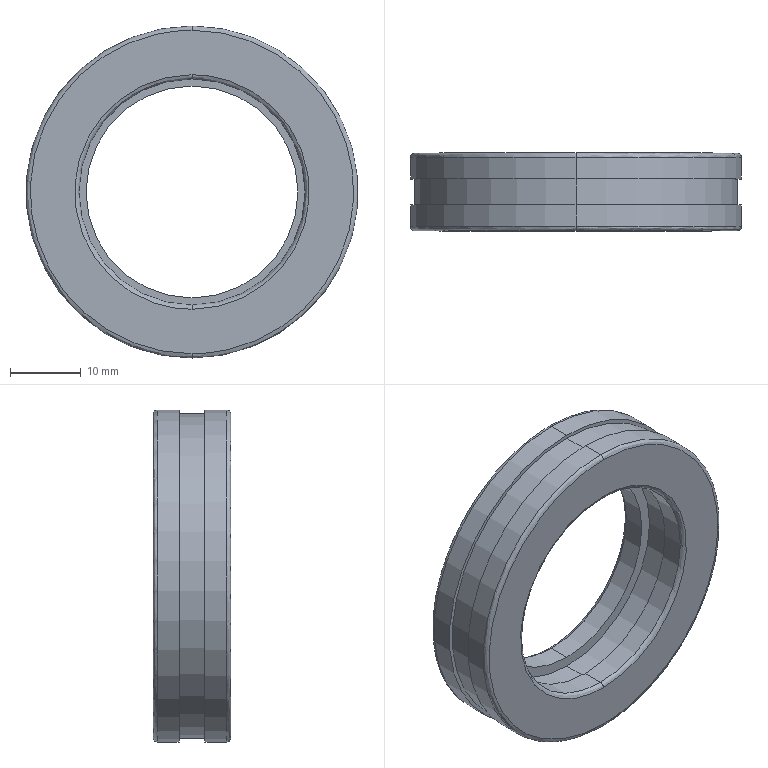Part | SolidWorks | features BaseBody 1 | 1 solid | 26 faces | box 47 x 11 x 47 mm | volume 10056 mm3 | cylinder 12 | spline 8 | plane 6 | commonest cylinder face diameters 47 x4 30 x2 32 x2 33.1 x2 45.9 x2
STEP:
#1=CARTESIAN_POINT('',(0.,10.4,-23.5));
#2=VERTEX_POINT('',#1);
#3=CARTESIAN_POINT('',(0.,10.4,23.5));
#4=VERTEX_POINT('',#3);
#5=CARTESIAN_POINT('',(0.,10.4,0.));
#6=DIRECTION('',(0.,1.,0.));
#7=DIRECTION('',(0.,0.,-1.));
#8=AXIS2_PLACEMENT_3D('',#5,#6,#7);
#9=CIRCLE('',#8,23.5);
#10=EDGE_CURVE('',#2,#4,#9,.T.);
#11=ORIENTED_EDGE('',*,*,#10,.T.);
#12=CARTESIAN_POINT('',(0.,11.,22.9));
#13=VERTEX_POINT('',#12);
#14=CARTESIAN_POINT('',(0.,10.4,22.9));
#15=DIRECTION('',(-1.,0.,0.));
#16=DIRECTION('',(0.,0.,1.));
#17=AXIS2_PLACEMENT_3D('',#14,#15,#16);
#18=CIRCLE('',#17,0.6);
#19=EDGE_CURVE('',#4,#13,#18,.T.);
#20=ORIENTED_EDGE('',*,*,#19,.T.);
#21=CARTESIAN_POINT('',(0.,11.,-22.9));
#22=VERTEX_POINT('',#21);
#23=CARTESIAN_POINT('',(0.,11.,-22.9));
#24=CARTESIAN_POINT('',(-0.7002,11.,-22.9));
#25=CARTESIAN_POINT('',(-1.746,11.,-22.852));
#26=CARTESIAN_POINT('',(-2.959,11.,-22.713));
#27=CARTESIAN_POINT('',(-3.564,11.,-22.622));
#28=CARTESIAN_POINT('',(-3.865,11.,-22.572));
#29=CARTESIAN_POINT('',(-4.016,11.,-22.545));
#30=CARTESIAN_POINT('',(-4.081,11.,-22.533));
#31=CARTESIAN_POINT('',(-4.124,11.,-22.526));
#32=CARTESIAN_POINT('',(-4.144,11.,-22.522));
#33=CARTESIAN_POINT('',(-4.897,11.,-22.383));
#34=CARTESIAN_POINT('',(-5.977,11.,-22.128));
#35=CARTESIAN_POINT('',(-7.212,11.,-21.74));
#36=CARTESIAN_POINT('',(-7.823,11.,-21.524));
#37=CARTESIAN_POINT('',(-8.127,11.,-21.41));
#38=CARTESIAN_POINT('',(-8.257,11.,-21.36));
#39=CARTESIAN_POINT('',(-8.343,11.,-21.326));
#40=CARTESIAN_POINT('',(-8.384,11.,-21.31));
#41=CARTESIAN_POINT('',(-9.149,11.,-21.007));
#42=CARTESIAN_POINT('',(-10.201,11.,-20.528));
#43=CARTESIAN_POINT('',(-11.382,11.,-19.878));
#44=CARTESIAN_POINT('',(-11.96,11.,-19.53));
#45=CARTESIAN_POINT('',(-12.206,11.,-19.376));
#46=CARTESIAN_POINT('',(-12.369,11.,-19.273));
#47=CARTESIAN_POINT('',(-12.448,11.,-19.221));
#48=CARTESIAN_POINT('',(-13.854,11.,-18.302));
#49=CARTESIAN_POINT('',(-15.075,11.,-17.31));
#50=CARTESIAN_POINT('',(-16.752,11.,-15.634));
#51=CARTESIAN_POINT('',(-17.542,11.,-14.757));
#52=CARTESIAN_POINT('',(-18.382,11.,-13.667));
#53=CARTESIAN_POINT('',(-18.782,11.,-13.105));
#54=CARTESIAN_POINT('',(-18.948,11.,-12.86));
#55=CARTESIAN_POINT('',(-19.059,11.,-12.696));
#56=CARTESIAN_POINT('',(-19.114,11.,-12.612));
#57=CARTESIAN_POINT('',(-19.591,11.,-11.884));
#58=CARTESIAN_POINT('',(-20.174,11.,-10.885));
#59=CARTESIAN_POINT('',(-20.763,11.,-9.673));
#60=CARTESIAN_POINT('',(-21.035,11.,-9.055));
#61=CARTESIAN_POINT('',(-21.166,11.,-8.743));
#62=CARTESIAN_POINT('',(-21.22,11.,-8.609));
#63=CARTESIAN_POINT('',(-21.256,11.,-8.519));
#64=CARTESIAN_POINT('',(-21.275,11.,-8.473));
#65=CARTESIAN_POINT('',(-21.565,11.,-7.739));
#66=CARTESIAN_POINT('',(-21.924,11.,-6.688));
#67=CARTESIAN_POINT('',(-22.251,11.,-5.436));
#68=CARTESIAN_POINT('',(-22.392,11.,-4.804));
#69=CARTESIAN_POINT('',(-22.457,11.,-4.486));
#70=CARTESIAN_POINT('',(-22.488,11.,-4.327));
#71=CARTESIAN_POINT('',(-22.501,11.,-4.258));
#72=CARTESIAN_POINT('',(-22.509,11.,-4.213));
#73=CARTESIAN_POINT('',(-22.514,11.,-4.188));
#74=CARTESIAN_POINT('',(-22.773,11.,-2.79));
#75=CARTESIAN_POINT('',(-22.9,11.,-1.4));
#76=CARTESIAN_POINT('',(-22.9,11.,0.7002));
#77=CARTESIAN_POINT('',(-22.852,11.,1.746));
#78=CARTESIAN_POINT('',(-22.713,11.,2.959));
#79=CARTESIAN_POINT('',(-22.622,11.,3.564));
#80=CARTESIAN_POINT('',(-22.572,11.,3.865));
#81=CARTESIAN_POINT('',(-22.545,11.,4.016));
#82=CARTESIAN_POINT('',(-22.533,11.,4.081));
#83=CARTESIAN_POINT('',(-22.526,11.,4.124));
#84=CARTESIAN_POINT('',(-22.522,11.,4.144));
#85=CARTESIAN_POINT('',(-22.383,11.,4.897));
#86=CARTESIAN_POINT('',(-22.128,11.,5.977));
#87=CARTESIAN_POINT('',(-21.74,11.,7.212));
#88=CARTESIAN_POINT('',(-21.524,11.,7.823));
#89=CARTESIAN_POINT('',(-21.41,11.,8.127));
#90=CARTESIAN_POINT('',(-21.36,11.,8.257));
#91=CARTESIAN_POINT('',(-21.326,11.,8.343));
#92=CARTESIAN_POINT('',(-21.31,11.,8.384));
#93=CARTESIAN_POINT('',(-21.007,11.,9.149));
#94=CARTESIAN_POINT('',(-20.528,11.,10.201));
#95=CARTESIAN_POINT('',(-19.878,11.,11.382));
#96=CARTESIAN_POINT('',(-19.53,11.,11.96));
#97=CARTESIAN_POINT('',(-19.376,11.,12.206));
#98=CARTESIAN_POINT('',(-19.273,11.,12.369));
#99=CARTESIAN_POINT('',(-19.221,11.,12.448));
#100=CARTESIAN_POINT('',(-18.302,11.,13.854));
#101=CARTESIAN_POINT('',(-17.31,11.,15.075));
#102=CARTESIAN_POINT('',(-15.634,11.,16.752));
#103=CARTESIAN_POINT('',(-14.757,11.,17.542));
#104=CARTESIAN_POINT('',(-13.667,11.,18.382));
#105=CARTESIAN_POINT('',(-13.105,11.,18.782));
#106=CARTESIAN_POINT('',(-12.86,11.,18.948));
#107=CARTESIAN_POINT('',(-12.696,11.,19.059));
#108=CARTESIAN_POINT('',(-12.612,11.,19.114));
#109=CARTESIAN_POINT('',(-11.884,11.,19.591));
#110=CARTESIAN_POINT('',(-10.885,11.,20.174));
#111=CARTESIAN_POINT('',(-9.673,11.,20.763));
#112=CARTESIAN_POINT('',(-9.055,11.,21.035));
#113=CARTESIAN_POINT('',(-8.743,11.,21.166));
#114=CARTESIAN_POINT('',(-8.609,11.,21.22));
#115=CARTESIAN_POINT('',(-8.519,11.,21.256));
#116=CARTESIAN_POINT('',(-8.473,11.,21.275));
#117=CARTESIAN_POINT('',(-7.739,11.,21.565));
#118=CARTESIAN_POINT('',(-6.688,11.,21.924));
#119=CARTESIAN_POINT('',(-5.436,11.,22.251));
#120=CARTESIAN_POINT('',(-4.804,11.,22.392));
#121=CARTESIAN_POINT('',(-4.486,11.,22.457));
#122=CARTESIAN_POINT('',(-4.327,11.,22.488));
#123=CARTESIAN_POINT('',(-4.258,11.,22.501));
#124=CARTESIAN_POINT('',(-4.213,11.,22.509));
#125=CARTESIAN_POINT('',(-4.188,11.,22.514));
#126=CARTESIAN_POINT('',(-2.79,11.,22.773));
#127=CARTESIAN_POINT('',(-1.4,11.,22.9));
#128=CARTESIAN_POINT('',(0.,11.,22.9));
#129=B_SPLINE_CURVE_WITH_KNOTS('',3,(#23,#24,#25,#26,#27,#28,#29,#30,#31,#32,#33,#34,#35,#36,#37,#38,#39,#40,#41,#42,#43,#44,#45,#46,#47,#48,#49,#50,#51,#52,#53,#54,#55,#56,#57,#58,#59,#60,#61,#62,#63,#64,#65,#66,#67,#68,#69,#70,#71,#72,#73,#74,#75,#76,#77,#78,#79,#80,#81,#82,#83,#84,#85,#86,#87,#88,#89,#90,#91,#92,#93,#94,#95,#96,#97,#98,#99,#100,#101,#102,#103,#104,#105,#106,#107,#108,#109,#110,#111,#112,#113,#114,#115,#116,#117,#118,#119,#120,#121,#122,#123,#124,#125,#126,#127,#128),.UNSPECIFIED.,.F.,.F.,(4,1,1,1,1,1,2,2,1,1,1,1,2,2,1,1,1,2,2,2,1,1,1,2,2,1,1,1,1,2,2,1,1,1,1,1,2,2,2,1,1,1,1,1,2,2,1,1,1,1,2,2,1,1,1,2,2,2,1,1,1,2,2,1,1,1,1,2,2,1,1,1,1,1,2,2,4),(0.,0.01563,0.02344,0.02734,0.0293,0.03027,0.03076,0.03125,0.04688,0.05469,0.05859,0.06055,0.06152,0.0625,0.07813,0.08594,0.08984,0.0918,0.09375,0.125,0.1406,0.1484,0.1523,0.1543,0.1563,0.1719,0.1797,0.1836,0.1855,0.1865,0.1875,0.2031,0.2109,0.2148,0.2168,0.2178,0.2183,0.2188,0.25,0.2656,0.2734,0.2773,0.2793,0.2803,0.2808,0.2813,0.2969,0.3047,0.3086,0.3105,0.3115,0.3125,0.3281,0.3359,0.3398,0.3418,0.3438,0.375,0.3906,0.3984,0.4023,0.4043,0.4063,0.4219,0.4297,0.4336,0.4355,0.4365,0.4375,0.4531,0.4609,0.4648,0.4668,0.4678,0.4683,0.4688,0.5),.UNSPECIFIED.);
#130=EDGE_CURVE('',#22,#13,#129,.T.);
#131=ORIENTED_EDGE('',*,*,#130,.F.);
#132=CARTESIAN_POINT('',(0.,10.4,-22.9));
#133=DIRECTION('',(1.,0.,0.));
#134=DIRECTION('',(0.,0.,-1.));
#135=AXIS2_PLACEMENT_3D('',#132,#133,#134);
#136=CIRCLE('',#135,0.6);
#137=EDGE_CURVE('',#2,#22,#136,.T.);
#138=ORIENTED_EDGE('',*,*,#137,.F.);
#139=EDGE_LOOP('',(#11,#20,#131,#138));
#140=FACE_OUTER_BOUND('',#139,.T.);
#141=CARTESIAN_POINT('',(0.,10.4,23.5));
#142=CARTESIAN_POINT('',(-47.,10.4,23.5));
#143=CARTESIAN_POINT('',(-47.,10.4,-23.5));
#144=CARTESIAN_POINT('',(0.,10.4,-23.5));
#145=CARTESIAN_POINT('',(0.,10.751,23.5));
#146=CARTESIAN_POINT('',(-47.,10.751,23.5));
#147=CARTESIAN_POINT('',(-47.,10.751,-23.5));
#148=CARTESIAN_POINT('',(0.,10.751,-23.5));
#149=CARTESIAN_POINT('',(0.,11.,23.251));
#150=CARTESIAN_POINT('',(-46.503,11.,23.251));
#151=CARTESIAN_POINT('',(-46.503,11.,-23.251));
#152=CARTESIAN_POINT('',(0.,11.,-23.251));
#153=CARTESIAN_POINT('',(0.,11.,22.9));
#154=CARTESIAN_POINT('',(-45.8,11.,22.9));
#155=CARTESIAN_POINT('',(-45.8,11.,-22.9));
#156=CARTESIAN_POINT('',(0.,11.,-22.9));
#157=(BOUNDED_SURFACE()B_SPLINE_SURFACE(3,3,((#141,#142,#143,#144),(#145,#146,#147,#148),(#149,#150,#151,#152),(#153,#154,#155,#156)),.UNSPECIFIED.,.F.,.F.,.F.)B_SPLINE_SURFACE_WITH_KNOTS((4,4),(4,4),(0.,1.),(0.,1.),.UNSPECIFIED.)GEOMETRIC_REPRESENTATION_ITEM()RATIONAL_B_SPLINE_SURFACE(((1.,0.3333,0.3333,1.),(0.8047,0.2682,0.2682,0.8047),(0.8047,0.2682,0.2682,0.8047),(1.,0.3333,0.3333,1.)))REPRESENTATION_ITEM('')SURFACE());
#158=ADVANCED_FACE('',(#140),#157,.T.);
#159=CARTESIAN_POINT('',(0.,11.,15.6));
#160=VERTEX_POINT('',#159);
#161=CARTESIAN_POINT('',(0.,11.,-15.6));
#162=VERTEX_POINT('',#161);
#163=CARTESIAN_POINT('',(0.,11.,15.6));
#164=CARTESIAN_POINT('',(-0.4769,11.,15.6));
#165=CARTESIAN_POINT('',(-1.189,11.,15.567));
#166=CARTESIAN_POINT('',(-2.016,11.,15.473));
#167=CARTESIAN_POINT('',(-2.428,11.,15.411));
#168=CARTESIAN_POINT('',(-2.633,11.,15.376));
#169=CARTESIAN_POINT('',(-2.721,11.,15.361));
#170=CARTESIAN_POINT('',(-2.78,11.,15.35));
#171=CARTESIAN_POINT('',(-2.808,11.,15.345));
#172=CARTESIAN_POINT('',(-3.336,11.,15.248));
#173=CARTESIAN_POINT('',(-4.072,11.,15.074));
#174=CARTESIAN_POINT('',(-4.913,11.,14.81));
#175=CARTESIAN_POINT('',(-5.329,11.,14.663));
#176=CARTESIAN_POINT('',(-5.536,11.,14.585));
#177=CARTESIAN_POINT('',(-5.625,11.,14.551));
#178=CARTESIAN_POINT('',(-5.683,11.,14.528));
#179=CARTESIAN_POINT('',(-5.712,11.,14.517));
#180=CARTESIAN_POINT('',(-6.232,11.,14.311));
#181=CARTESIAN_POINT('',(-6.949,11.,13.984));
#182=CARTESIAN_POINT('',(-7.753,11.,13.541));
#183=CARTESIAN_POINT('',(-8.148,11.,13.304));
#184=CARTESIAN_POINT('',(-8.315,11.,13.2));
#185=CARTESIAN_POINT('',(-8.426,11.,13.129));
#186=CARTESIAN_POINT('',(-8.48,11.,13.094));
#187=CARTESIAN_POINT('',(-9.438,11.,12.468));
#188=CARTESIAN_POINT('',(-10.27,11.,11.792));
#189=CARTESIAN_POINT('',(-11.412,11.,10.65));
#190=CARTESIAN_POINT('',(-11.95,11.,10.053));
#191=CARTESIAN_POINT('',(-12.522,11.,9.31));
#192=CARTESIAN_POINT('',(-12.795,11.,8.927));
#193=CARTESIAN_POINT('',(-12.908,11.,8.761));
#194=CARTESIAN_POINT('',(-12.983,11.,8.649));
#195=CARTESIAN_POINT('',(-13.021,11.,8.592));
#196=CARTESIAN_POINT('',(-13.346,11.,8.095));
#197=CARTESIAN_POINT('',(-13.743,11.,7.415));
#198=CARTESIAN_POINT('',(-14.144,11.,6.59));
#199=CARTESIAN_POINT('',(-14.33,11.,6.169));
#200=CARTESIAN_POINT('',(-14.418,11.,5.956));
#201=CARTESIAN_POINT('',(-14.456,11.,5.865));
#202=CARTESIAN_POINT('',(-14.48,11.,5.804));
#203=CARTESIAN_POINT('',(-14.493,11.,5.772));
#204=CARTESIAN_POINT('',(-14.691,11.,5.272));
#205=CARTESIAN_POINT('',(-14.935,11.,4.556));
#206=CARTESIAN_POINT('',(-15.158,11.,3.704));
#207=CARTESIAN_POINT('',(-15.254,11.,3.273));
#208=CARTESIAN_POINT('',(-15.298,11.,3.056));
#209=CARTESIAN_POINT('',(-15.316,11.,2.963));
#210=CARTESIAN_POINT('',(-15.328,11.,2.901));
#211=CARTESIAN_POINT('',(-15.334,11.,2.868));
#212=CARTESIAN_POINT('',(-15.513,11.,1.901));
#213=CARTESIAN_POINT('',(-15.6,11.,0.9538));
#214=CARTESIAN_POINT('',(-15.6,11.,-0.4769));
#215=CARTESIAN_POINT('',(-15.567,11.,-1.189));
#216=CARTESIAN_POINT('',(-15.473,11.,-2.016));
#217=CARTESIAN_POINT('',(-15.411,11.,-2.428));
#218=CARTESIAN_POINT('',(-15.376,11.,-2.633));
#219=CARTESIAN_POINT('',(-15.361,11.,-2.721));
#220=CARTESIAN_POINT('',(-15.35,11.,-2.78));
#221=CARTESIAN_POINT('',(-15.345,11.,-2.808));
#222=CARTESIAN_POINT('',(-15.248,11.,-3.336));
#223=CARTESIAN_POINT('',(-15.074,11.,-4.072));
#224=CARTESIAN_POINT('',(-14.81,11.,-4.913));
#225=CARTESIAN_POINT('',(-14.663,11.,-5.329));
#226=CARTESIAN_POINT('',(-14.585,11.,-5.536));
#227=CARTESIAN_POINT('',(-14.551,11.,-5.625));
#228=CARTESIAN_POINT('',(-14.528,11.,-5.683));
#229=CARTESIAN_POINT('',(-14.517,11.,-5.712));
#230=CARTESIAN_POINT('',(-14.311,11.,-6.232));
#231=CARTESIAN_POINT('',(-13.984,11.,-6.949));
#232=CARTESIAN_POINT('',(-13.541,11.,-7.753));
#233=CARTESIAN_POINT('',(-13.304,11.,-8.148));
#234=CARTESIAN_POINT('',(-13.2,11.,-8.315));
#235=CARTESIAN_POINT('',(-13.129,11.,-8.426));
#236=CARTESIAN_POINT('',(-13.094,11.,-8.48));
#237=CARTESIAN_POINT('',(-12.468,11.,-9.438));
#238=CARTESIAN_POINT('',(-11.792,11.,-10.27));
#239=CARTESIAN_POINT('',(-10.65,11.,-11.412));
#240=CARTESIAN_POINT('',(-10.053,11.,-11.95));
#241=CARTESIAN_POINT('',(-9.31,11.,-12.522));
#242=CARTESIAN_POINT('',(-8.927,11.,-12.795));
#243=CARTESIAN_POINT('',(-8.761,11.,-12.908));
#244=CARTESIAN_POINT('',(-8.649,11.,-12.983));
#245=CARTESIAN_POINT('',(-8.592,11.,-13.021));
#246=CARTESIAN_POINT('',(-8.095,11.,-13.346));
#247=CARTESIAN_POINT('',(-7.415,11.,-13.743));
#248=CARTESIAN_POINT('',(-6.59,11.,-14.144));
#249=CARTESIAN_POINT('',(-6.169,11.,-14.33));
#250=CARTESIAN_POINT('',(-5.956,11.,-14.418));
#251=CARTESIAN_POINT('',(-5.865,11.,-14.456));
#252=CARTESIAN_POINT('',(-5.804,11.,-14.48));
#253=CARTESIAN_POINT('',(-5.772,11.,-14.493));
#254=CARTESIAN_POINT('',(-5.272,11.,-14.691));
#255=CARTESIAN_POINT('',(-4.556,11.,-14.935));
#256=CARTESIAN_POINT('',(-3.704,11.,-15.158));
#257=CARTESIAN_POINT('',(-3.273,11.,-15.254));
#258=CARTESIAN_POINT('',(-3.056,11.,-15.298));
#259=CARTESIAN_POINT('',(-2.963,11.,-15.316));
#260=CARTESIAN_POINT('',(-2.901,11.,-15.328));
#261=CARTESIAN_POINT('',(-2.868,11.,-15.334));
#262=CARTESIAN_POINT('',(-1.901,11.,-15.513));
#263=CARTESIAN_POINT('',(-0.9544,11.,-15.6));
#264=CARTESIAN_POINT('',(0.,11.,-15.6));
#265=B_SPLINE_CURVE_WITH_KNOTS('',3,(#163,#164,#165,#166,#167,#168,#169,#170,#171,#172,#173,#174,#175,#176,#177,#178,#179,#180,#181,#182,#183,#184,#185,#186,#187,#188,#189,#190,#191,#192,#193,#194,#195,#196,#197,#198,#199,#200,#201,#202,#203,#204,#205,#206,#207,#208,#209,#210,#211,#212,#213,#214,#215,#216,#217,#218,#219,#220,#221,#222,#223,#224,#225,#226,#227,#228,#229,#230,#231,#232,#233,#234,#235,#236,#237,#238,#239,#240,#241,#242,#243,#244,#245,#246,#247,#248,#249,#250,#251,#252,#253,#254,#255,#256,#257,#258,#259,#260,#261,#262,#263,#264),.UNSPECIFIED.,.F.,.F.,(4,1,1,1,1,2,2,1,1,1,1,2,2,1,1,1,2,2,2,1,1,1,2,2,1,1,1,1,2,2,1,1,1,1,2,2,2,1,1,1,1,2,2,1,1,1,1,2,2,1,1,1,2,2,2,1,1,1,2,2,1,1,1,1,2,2,1,1,1,1,2,2,4),(0.5,0.5156,0.5234,0.5273,0.5293,0.5303,0.5313,0.5469,0.5547,0.5586,0.5605,0.5615,0.5625,0.5781,0.5859,0.5898,0.5918,0.5938,0.625,0.6406,0.6484,0.6523,0.6543,0.6563,0.6719,0.6797,0.6836,0.6855,0.6865,0.6875,0.7031,0.7109,0.7148,0.7168,0.7178,0.7188,0.75,0.7656,0.7734,0.7773,0.7793,0.7803,0.7813,0.7969,0.8047,0.8086,0.8105,0.8115,0.8125,0.8281,0.8359,0.8398,0.8418,0.8438,0.875,0.8906,0.8984,0.9023,0.9043,0.9063,0.9219,0.9297,0.9336,0.9355,0.9365,0.9375,0.9531,0.9609,0.9648,0.9668,0.9678,0.9688,1.),.UNSPECIFIED.);
#266=EDGE_CURVE('',#160,#162,#265,.T.);
#267=ORIENTED_EDGE('',*,*,#266,.F.);
#268=CARTESIAN_POINT('',(0.,10.4,15.));
#269=VERTEX_POINT('',#268);
#270=CARTESIAN_POINT('',(0.,10.4,15.6));
#271=DIRECTION('',(-1.,0.,0.));
#272=DIRECTION('',(0.,0.,1.));
#273=AXIS2_PLACEMENT_3D('',#270,#271,#272);
#274=CIRCLE('',#273,0.6);
#275=EDGE_CURVE('',#160,#269,#274,.T.);
#276=ORIENTED_EDGE('',*,*,#275,.T.);
#277=CARTESIAN_POINT('',(0.,10.4,-15.));
#278=VERTEX_POINT('',#277);
#279=CARTESIAN_POINT('',(0.,10.4,0.));
#280=DIRECTION('',(0.,-1.,0.));
#281=DIRECTION('',(0.,0.,-1.));
#282=AXIS2_PLACEMENT_3D('',#279,#280,#281);
#283=CIRCLE('',#282,15.);
#284=EDGE_CURVE('',#269,#278,#283,.T.);
#285=ORIENTED_EDGE('',*,*,#284,.T.);
#286=CARTESIAN_POINT('',(0.,10.4,-15.6));
#287=DIRECTION('',(1.,0.,0.));
#288=DIRECTION('',(0.,0.,-1.));
#289=AXIS2_PLACEMENT_3D('',#286,#287,#288);
#290=CIRCLE('',#289,0.6);
#291=EDGE_CURVE('',#162,#278,#290,.T.);
#292=ORIENTED_EDGE('',*,*,#291,.F.);
#293=EDGE_LOOP('',(#267,#276,#285,#292));
#294=FACE_OUTER_BOUND('',#293,.T.);
#295=CARTESIAN_POINT('',(0.,11.,15.6));
#296=CARTESIAN_POINT('',(-31.2,11.,15.6));
#297=CARTESIAN_POINT('',(-31.2,11.,-15.6));
#298=CARTESIAN_POINT('',(0.,11.,-15.6));
#299=CARTESIAN_POINT('',(0.,11.,15.249));
#300=CARTESIAN_POINT('',(-30.497,11.,15.249));
#301=CARTESIAN_POINT('',(-30.497,11.,-15.249));
#302=CARTESIAN_POINT('',(0.,11.,-15.249));
#303=CARTESIAN_POINT('',(0.,10.751,15.));
#304=CARTESIAN_POINT('',(-30.,10.751,15.));
#305=CARTESIAN_POINT('',(-30.,10.751,-15.));
#306=CARTESIAN_POINT('',(0.,10.751,-15.));
#307=CARTESIAN_POINT('',(0.,10.4,15.));
#308=CARTESIAN_POINT('',(-30.,10.4,15.));
#309=CARTESIAN_POINT('',(-30.,10.4,-15.));
#310=CARTESIAN_POINT('',(0.,10.4,-15.));
#311=(BOUNDED_SURFACE()B_SPLINE_SURFACE(3,3,((#295,#296,#297,#298),(#299,#300,#301,#302),(#303,#304,#305,#306),(#307,#308,#309,#310)),.UNSPECIFIED.,.F.,.F.,.F.)B_SPLINE_SURFACE_WITH_KNOTS((4,4),(4,4),(0.,1.),(0.,1.),.UNSPECIFIED.)GEOMETRIC_REPRESENTATION_ITEM()RATIONAL_B_SPLINE_SURFACE(((1.,0.3333,0.3333,1.),(0.8047,0.2682,0.2682,0.8047),(0.8047,0.2682,0.2682,0.8047),(1.,0.3333,0.3333,1.)))REPRESENTATION_ITEM('')SURFACE());
#312=ADVANCED_FACE('',(#294),#311,.T.);
#313=CARTESIAN_POINT('',(0.,0.,-22.9));
#314=VERTEX_POINT('',#313);
#315=CARTESIAN_POINT('',(0.,0.,22.9));
#316=VERTEX_POINT('',#315);
#317=CARTESIAN_POINT('',(0.,0.,-22.9));
#318=CARTESIAN_POINT('',(-45.8,0.,-22.9));
#319=CARTESIAN_POINT('',(-45.8,0.,22.9));
#320=CARTESIAN_POINT('',(0.,0.,22.9));
#321=(BOUNDED_CURVE()B_SPLINE_CURVE(3,(#317,#318,#319,#320),.UNSPECIFIED.,.F.,.F.)B_SPLINE_CURVE_WITH_KNOTS((4,4),(0.,0.5),.UNSPECIFIED.)CURVE()GEOMETRIC_REPRESENTATION_ITEM()RATIONAL_B_SPLINE_CURVE((1.,0.3333,0.3333,1.))REPRESENTATION_ITEM(''));
#322=EDGE_CURVE('',#314,#316,#321,.T.);
#323=ORIENTED_EDGE('',*,*,#322,.T.);
#324=CARTESIAN_POINT('',(0.,0.6,23.5));
#325=VERTEX_POINT('',#324);
#326=CARTESIAN_POINT('',(0.,0.6,22.9));
#327=DIRECTION('',(-1.,0.,0.));
#328=DIRECTION('',(0.,0.,1.));
#329=AXIS2_PLACEMENT_3D('',#326,#327,#328);
#330=CIRCLE('',#329,0.6);
#331=EDGE_CURVE('',#316,#325,#330,.T.);
#332=ORIENTED_EDGE('',*,*,#331,.T.);
#333=CARTESIAN_POINT('',(0.,0.6,-23.5));
#334=VERTEX_POINT('',#333);
#335=CARTESIAN_POINT('',(0.,0.6,0.));
#336=DIRECTION('',(0.,1.,0.));
#337=DIRECTION('',(0.,0.,1.));
#338=AXIS2_PLACEMENT_3D('',#335,#336,#337);
#339=CIRCLE('',#338,23.5);
#340=EDGE_CURVE('',#334,#325,#339,.T.);
#341=ORIENTED_EDGE('',*,*,#340,.F.);
#342=CARTESIAN_POINT('',(0.,0.6,-22.9));
#343=DIRECTION('',(1.,0.,0.));
#344=DIRECTION('',(0.,0.,-1.));
#345=AXIS2_PLACEMENT_3D('',#342,#343,#344);
#346=CIRCLE('',#345,0.6);
#347=EDGE_CURVE('',#314,#334,#346,.T.);
#348=ORIENTED_EDGE('',*,*,#347,.F.);
#349=EDGE_LOOP('',(#323,#332,#341,#348));
#350=FACE_OUTER_BOUND('',#349,.T.);
#351=CARTESIAN_POINT('',(0.,0.,22.9));
#352=CARTESIAN_POINT('',(-45.8,0.,22.9));
#353=CARTESIAN_POINT('',(-45.8,0.,-22.9));
#354=CARTESIAN_POINT('',(0.,0.,-22.9));
#355=CARTESIAN_POINT('',(0.,0.,23.251));
#356=CARTESIAN_POINT('',(-46.503,0.,23.251));
#357=CARTESIAN_POINT('',(-46.503,0.,-23.251));
#358=CARTESIAN_POINT('',(0.,0.,-23.251));
#359=CARTESIAN_POINT('',(0.,0.2485,23.5));
#360=CARTESIAN_POINT('',(-47.,0.2485,23.5));
#361=CARTESIAN_POINT('',(-47.,0.2485,-23.5));
#362=CARTESIAN_POINT('',(0.,0.2485,-23.5));
#363=CARTESIAN_POINT('',(0.,0.6,23.5));
#364=CARTESIAN_POINT('',(-47.,0.6,23.5));
#365=CARTESIAN_POINT('',(-47.,0.6,-23.5));
#366=CARTESIAN_POINT('',(0.,0.6,-23.5));
#367=(BOUNDED_SURFACE()B_SPLINE_SURFACE(3,3,((#351,#352,#353,#354),(#355,#356,#357,#358),(#359,#360,#361,#362),(#363,#364,#365,#366)),.UNSPECIFIED.,.F.,.F.,.F.)B_SPLINE_SURFACE_WITH_KNOTS((4,4),(4,4),(0.,1.),(0.,1.),.UNSPECIFIED.)GEOMETRIC_REPRESENTATION_ITEM()RATIONAL_B_SPLINE_SURFACE(((1.,0.3333,0.3333,1.),(0.8047,0.2682,0.2682,0.8047),(0.8047,0.2682,0.2682,0.8047),(1.,0.3333,0.3333,1.)))REPRESENTATION_ITEM('')SURFACE());
#368=ADVANCED_FACE('',(#350),#367,.T.);
#369=CARTESIAN_POINT('',(0.,0.6,-16.));
#370=VERTEX_POINT('',#369);
#371=CARTESIAN_POINT('',(0.,0.6,16.));
#372=VERTEX_POINT('',#371);
#373=CARTESIAN_POINT('',(0.,0.6,0.));
#374=DIRECTION('',(0.,1.,0.));
#375=DIRECTION('',(0.,0.,1.));
#376=AXIS2_PLACEMENT_3D('',#373,#374,#375);
#377=CIRCLE('',#376,16.);
#378=EDGE_CURVE('',#370,#372,#377,.T.);
#379=ORIENTED_EDGE('',*,*,#378,.T.);
#380=CARTESIAN_POINT('',(0.,0.,16.6));
#381=VERTEX_POINT('',#380);
#382=CARTESIAN_POINT('',(0.,0.6,16.6));
#383=DIRECTION('',(-1.,0.,0.));
#384=DIRECTION('',(0.,0.,1.));
#385=AXIS2_PLACEMENT_3D('',#382,#383,#384);
#386=CIRCLE('',#385,0.6);
#387=EDGE_CURVE('',#372,#381,#386,.T.);
#388=ORIENTED_EDGE('',*,*,#387,.T.);
#389=CARTESIAN_POINT('',(0.,0.,-16.6));
#390=VERTEX_POINT('',#389);
#391=CARTESIAN_POINT('',(0.,0.,16.6));
#392=CARTESIAN_POINT('',(-33.2,0.,16.6));
#393=CARTESIAN_POINT('',(-33.2,0.,-16.6));
#394=CARTESIAN_POINT('',(0.,0.,-16.6));
#395=(BOUNDED_CURVE()B_SPLINE_CURVE(3,(#391,#392,#393,#394),.UNSPECIFIED.,.F.,.F.)B_SPLINE_CURVE_WITH_KNOTS((4,4),(0.5,1.),.UNSPECIFIED.)CURVE()GEOMETRIC_REPRESENTATION_ITEM()RATIONAL_B_SPLINE_CURVE((1.,0.3333,0.3333,1.))REPRESENTATION_ITEM(''));
#396=EDGE_CURVE('',#381,#390,#395,.T.);
#397=ORIENTED_EDGE('',*,*,#396,.T.);
#398=CARTESIAN_POINT('',(0.,0.6,-16.6));
#399=DIRECTION('',(1.,0.,0.));
#400=DIRECTION('',(0.,0.,-1.));
#401=AXIS2_PLACEMENT_3D('',#398,#399,#400);
#402=CIRCLE('',#401,0.6);
#403=EDGE_CURVE('',#370,#390,#402,.T.);
#404=ORIENTED_EDGE('',*,*,#403,.F.);
#405=EDGE_LOOP('',(#379,#388,#397,#404));
#406=FACE_OUTER_BOUND('',#405,.T.);
#407=CARTESIAN_POINT('',(0.,0.6,16.));
#408=CARTESIAN_POINT('',(-32.,0.6,16.));
#409=CARTESIAN_POINT('',(-32.,0.6,-16.));
#410=CARTESIAN_POINT('',(0.,0.6,-16.));
#411=CARTESIAN_POINT('',(0.,0.2485,16.));
#412=CARTESIAN_POINT('',(-32.,0.2485,16.));
#413=CARTESIAN_POINT('',(-32.,0.2485,-16.));
#414=CARTESIAN_POINT('',(0.,0.2485,-16.));
#415=CARTESIAN_POINT('',(0.,0.,16.249));
#416=CARTESIAN_POINT('',(-32.497,0.,16.249));
#417=CARTESIAN_POINT('',(-32.497,0.,-16.249));
#418=CARTESIAN_POINT('',(0.,0.,-16.249));
#419=CARTESIAN_POINT('',(0.,0.,16.6));
#420=CARTESIAN_POINT('',(-33.2,0.,16.6));
#421=CARTESIAN_POINT('',(-33.2,0.,-16.6));
#422=CARTESIAN_POINT('',(0.,0.,-16.6));
#423=(BOUNDED_SURFACE()B_SPLINE_SURFACE(3,3,((#407,#408,#409,#410),(#411,#412,#413,#414),(#415,#416,#417,#418),(#419,#420,#421,#422)),.UNSPECIFIED.,.F.,.F.,.F.)B_SPLINE_SURFACE_WITH_KNOTS((4,4),(4,4),(0.,1.),(0.,1.),.UNSPECIFIED.)GEOMETRIC_REPRESENTATION_ITEM()RATIONAL_B_SPLINE_SURFACE(((1.,0.3333,0.3333,1.),(0.8047,0.2682,0.2682,0.8047),(0.8047,0.2682,0.2682,0.8047),(1.,0.3333,0.3333,1.)))REPRESENTATION_ITEM('')SURFACE());
#424=ADVANCED_FACE('',(#406),#423,.T.);
#425=CARTESIAN_POINT('',(0.,7.333,23.5));
#426=VERTEX_POINT('',#425);
#427=CARTESIAN_POINT('',(0.,7.333,-23.5));
#428=VERTEX_POINT('',#427);
#429=CARTESIAN_POINT('',(0.,7.333,0.));
#430=DIRECTION('',(0.,1.,0.));
#431=DIRECTION('',(0.,0.,1.));
#432=AXIS2_PLACEMENT_3D('',#429,#430,#431);
#433=CIRCLE('',#432,23.5);
#434=EDGE_CURVE('',#426,#428,#433,.T.);
#435=ORIENTED_EDGE('',*,*,#434,.T.);
#436=CARTESIAN_POINT('',(0.,0.,-23.5));
#437=DIRECTION('',(0.,1.,0.));
#438=VECTOR('',#437,1000.);
#439=LINE('',#436,#438);
#440=EDGE_CURVE('',#428,#2,#439,.T.);
#441=ORIENTED_EDGE('',*,*,#440,.T.);
#442=CARTESIAN_POINT('',(0.,10.4,0.));
#443=DIRECTION('',(0.,1.,0.));
#444=DIRECTION('',(0.,0.,-1.));
#445=AXIS2_PLACEMENT_3D('',#442,#443,#444);
#446=CIRCLE('',#445,23.5);
#447=EDGE_CURVE('',#4,#2,#446,.T.);
#448=ORIENTED_EDGE('',*,*,#447,.F.);
#449=CARTESIAN_POINT('',(0.,0.,23.5));
#450=DIRECTION('',(0.,1.,0.));
#451=VECTOR('',#450,1000.);
#452=LINE('',#449,#451);
#453=EDGE_CURVE('',#426,#4,#452,.T.);
#454=ORIENTED_EDGE('',*,*,#453,.F.);
#455=EDGE_LOOP('',(#435,#441,#448,#454));
#456=FACE_OUTER_BOUND('',#455,.T.);
#457=CARTESIAN_POINT('',(0.,0.,0.));
#458=DIRECTION('',(0.,1.,0.));
#459=DIRECTION('',(0.,0.,1.));
#460=AXIS2_PLACEMENT_3D('',#457,#458,#459);
#461=CYLINDRICAL_SURFACE('',#460,23.5);
#462=ADVANCED_FACE('',(#456),#461,.T.);
#463=CARTESIAN_POINT('',(0.,7.333,-15.));
#464=VERTEX_POINT('',#463);
#465=CARTESIAN_POINT('',(0.,7.333,15.));
#466=VERTEX_POINT('',#465);
#467=CARTESIAN_POINT('',(0.,7.333,0.));
#468=DIRECTION('',(0.,1.,0.));
#469=DIRECTION('',(0.,0.,1.));
#470=AXIS2_PLACEMENT_3D('',#467,#468,#469);
#471=CIRCLE('',#470,15.);
#472=EDGE_CURVE('',#464,#466,#471,.T.);
#473=ORIENTED_EDGE('',*,*,#472,.F.);
#474=CARTESIAN_POINT('',(0.,0.,-15.));
#475=DIRECTION('',(0.,1.,0.));
#476=VECTOR('',#475,1000.);
#477=LINE('',#474,#476);
#478=EDGE_CURVE('',#464,#278,#477,.T.);
#479=ORIENTED_EDGE('',*,*,#478,.T.);
#480=ORIENTED_EDGE('',*,*,#284,.F.);
#481=CARTESIAN_POINT('',(0.,0.,15.));
#482=DIRECTION('',(0.,1.,0.));
#483=VECTOR('',#482,1000.);
#484=LINE('',#481,#483);
#485=EDGE_CURVE('',#466,#269,#484,.T.);
#486=ORIENTED_EDGE('',*,*,#485,.F.);
#487=EDGE_LOOP('',(#473,#479,#480,#486));
#488=FACE_OUTER_BOUND('',#487,.T.);
#489=CARTESIAN_POINT('',(0.,0.,0.));
#490=DIRECTION('',(0.,1.,0.));
#491=DIRECTION('',(0.,0.,1.));
#492=AXIS2_PLACEMENT_3D('',#489,#490,#491);
#493=CYLINDRICAL_SURFACE('',#492,15.);
#494=ADVANCED_FACE('',(#488),#493,.F.);
#495=CARTESIAN_POINT('',(0.,3.667,22.95));
#496=VERTEX_POINT('',#495);
#497=CARTESIAN_POINT('',(0.,3.667,-22.95));
#498=VERTEX_POINT('',#497);
#499=CARTESIAN_POINT('',(0.,3.667,0.));
#500=DIRECTION('',(0.,1.,0.));
#501=DIRECTION('',(0.,0.,1.));
#502=AXIS2_PLACEMENT_3D('',#499,#500,#501);
#503=CIRCLE('',#502,22.95);
#504=EDGE_CURVE('',#496,#498,#503,.T.);
#505=ORIENTED_EDGE('',*,*,#504,.T.);
#506=CARTESIAN_POINT('',(0.,7.333,-22.95));
#507=VERTEX_POINT('',#506);
#508=CARTESIAN_POINT('',(0.,0.,-22.95));
#509=DIRECTION('',(0.,1.,0.));
#510=VECTOR('',#509,1000.);
#511=LINE('',#508,#510);
#512=EDGE_CURVE('',#498,#507,#511,.T.);
#513=ORIENTED_EDGE('',*,*,#512,.T.);
#514=CARTESIAN_POINT('',(0.,7.333,22.95));
#515=VERTEX_POINT('',#514);
#516=CARTESIAN_POINT('',(0.,7.333,0.));
#517=DIRECTION('',(0.,1.,0.));
#518=DIRECTION('',(0.,0.,1.));
#519=AXIS2_PLACEMENT_3D('',#516,#517,#518);
#520=CIRCLE('',#519,22.95);
#521=EDGE_CURVE('',#515,#507,#520,.T.);
#522=ORIENTED_EDGE('',*,*,#521,.F.);
#523=CARTESIAN_POINT('',(0.,0.,22.95));
#524=DIRECTION('',(0.,1.,0.));
#525=VECTOR('',#524,1000.);
#526=LINE('',#523,#525);
#527=EDGE_CURVE('',#496,#515,#526,.T.);
#528=ORIENTED_EDGE('',*,*,#527,.F.);
#529=EDGE_LOOP('',(#505,#513,#522,#528));
#530=FACE_OUTER_BOUND('',#529,.T.);
#531=CARTESIAN_POINT('',(0.,0.,0.));
#532=DIRECTION('',(0.,1.,0.));
#533=DIRECTION('',(0.,0.,1.));
#534=AXIS2_PLACEMENT_3D('',#531,#532,#533);
#535=CYLINDRICAL_SURFACE('',#534,22.95);
#536=ADVANCED_FACE('',(#530),#535,.T.);
#537=CARTESIAN_POINT('',(0.,3.667,-16.55));
#538=VERTEX_POINT('',#537);
#539=CARTESIAN_POINT('',(0.,3.667,16.55));
#540=VERTEX_POINT('',#539);
#541=CARTESIAN_POINT('',(0.,3.667,0.));
#542=DIRECTION('',(0.,1.,0.));
#543=DIRECTION('',(0.,0.,1.));
#544=AXIS2_PLACEMENT_3D('',#541,#542,#543);
#545=CIRCLE('',#544,16.55);
#546=EDGE_CURVE('',#538,#540,#545,.T.);
#547=ORIENTED_EDGE('',*,*,#546,.F.);
#548=CARTESIAN_POINT('',(0.,7.333,-16.55));
#549=VERTEX_POINT('',#548);
#550=CARTESIAN_POINT('',(0.,0.,-16.55));
#551=DIRECTION('',(0.,1.,0.));
#552=VECTOR('',#551,1000.);
#553=LINE('',#550,#552);
#554=EDGE_CURVE('',#538,#549,#553,.T.);
#555=ORIENTED_EDGE('',*,*,#554,.T.);
#556=CARTESIAN_POINT('',(0.,7.333,16.55));
#557=VERTEX_POINT('',#556);
#558=CARTESIAN_POINT('',(0.,7.333,0.));
#559=DIRECTION('',(0.,-1.,0.));
#560=DIRECTION('',(0.,0.,1.));
#561=AXIS2_PLACEMENT_3D('',#558,#559,#560);
#562=CIRCLE('',#561,16.55);
#563=EDGE_CURVE('',#557,#549,#562,.T.);
#564=ORIENTED_EDGE('',*,*,#563,.F.);
#565=CARTESIAN_POINT('',(0.,0.,16.55));
#566=DIRECTION('',(0.,1.,0.));
#567=VECTOR('',#566,1000.);
#568=LINE('',#565,#567);
#569=EDGE_CURVE('',#540,#557,#568,.T.);
#570=ORIENTED_EDGE('',*,*,#569,.F.);
#571=EDGE_LOOP('',(#547,#555,#564,#570));
#572=FACE_OUTER_BOUND('',#571,.T.);
#573=CARTESIAN_POINT('',(0.,0.,0.));
#574=DIRECTION('',(0.,1.,0.));
#575=DIRECTION('',(0.,0.,1.));
#576=AXIS2_PLACEMENT_3D('',#573,#574,#575);
#577=CYLINDRICAL_SURFACE('',#576,16.55);
#578=ADVANCED_FACE('',(#572),#577,.F.);
#579=CARTESIAN_POINT('',(0.,0.6,0.));
#580=DIRECTION('',(0.,1.,0.));
#581=DIRECTION('',(0.,0.,1.));
#582=AXIS2_PLACEMENT_3D('',#579,#580,#581);
#583=CIRCLE('',#582,23.5);
#584=EDGE_CURVE('',#325,#334,#583,.T.);
#585=ORIENTED_EDGE('',*,*,#584,.T.);
#586=CARTESIAN_POINT('',(0.,3.667,-23.5));
#587=VERTEX_POINT('',#586);
#588=CARTESIAN_POINT('',(0.,0.,-23.5));
#589=DIRECTION('',(0.,1.,0.));
#590=VECTOR('',#589,1000.);
#591=LINE('',#588,#590);
#592=EDGE_CURVE('',#334,#587,#591,.T.);
#593=ORIENTED_EDGE('',*,*,#592,.T.);
#594=CARTESIAN_POINT('',(0.,3.667,23.5));
#595=VERTEX_POINT('',#594);
#596=CARTESIAN_POINT('',(0.,3.667,0.));
#597=DIRECTION('',(0.,1.,0.));
#598=DIRECTION('',(0.,0.,1.));
#599=AXIS2_PLACEMENT_3D('',#596,#597,#598);
#600=CIRCLE('',#599,23.5);
#601=EDGE_CURVE('',#595,#587,#600,.T.);
#602=ORIENTED_EDGE('',*,*,#601,.F.);
#603=CARTESIAN_POINT('',(0.,0.,23.5));
#604=DIRECTION('',(0.,1.,0.));
#605=VECTOR('',#604,1000.);
#606=LINE('',#603,#605);
#607=EDGE_CURVE('',#325,#595,#606,.T.);
#608=ORIENTED_EDGE('',*,*,#607,.F.);
#609=EDGE_LOOP('',(#585,#593,#602,#608));
#610=FACE_OUTER_BOUND('',#609,.T.);
#611=CARTESIAN_POINT('',(0.,0.,0.));
#612=DIRECTION('',(0.,1.,0.));
#613=DIRECTION('',(0.,0.,1.));
#614=AXIS2_PLACEMENT_3D('',#611,#612,#613);
#615=CYLINDRICAL_SURFACE('',#614,23.5);
#616=ADVANCED_FACE('',(#610),#615,.T.);
#617=ORIENTED_EDGE('',*,*,#378,.F.);
#618=CARTESIAN_POINT('',(0.,3.667,-16.));
#619=VERTEX_POINT('',#618);
#620=CARTESIAN_POINT('',(0.,0.,-16.));
#621=DIRECTION('',(0.,1.,0.));
#622=VECTOR('',#621,1000.);
#623=LINE('',#620,#622);
#624=EDGE_CURVE('',#370,#619,#623,.T.);
#625=ORIENTED_EDGE('',*,*,#624,.T.);
#626=CARTESIAN_POINT('',(0.,3.667,16.));
#627=VERTEX_POINT('',#626);
#628=CARTESIAN_POINT('',(0.,3.667,0.));
#629=DIRECTION('',(0.,-1.,0.));
#630=DIRECTION('',(0.,0.,1.));
#631=AXIS2_PLACEMENT_3D('',#628,#629,#630);
#632=CIRCLE('',#631,16.);
#633=EDGE_CURVE('',#627,#619,#632,.T.);
#634=ORIENTED_EDGE('',*,*,#633,.F.);
#635=CARTESIAN_POINT('',(0.,0.,16.));
#636=DIRECTION('',(0.,1.,0.));
#637=VECTOR('',#636,1000.);
#638=LINE('',#635,#637);
#639=EDGE_CURVE('',#372,#627,#638,.T.);
#640=ORIENTED_EDGE('',*,*,#639,.F.);
#641=EDGE_LOOP('',(#617,#625,#634,#640));
#642=FACE_OUTER_BOUND('',#641,.T.);
#643=CARTESIAN_POINT('',(0.,0.,0.));
#644=DIRECTION('',(0.,1.,0.));
#645=DIRECTION('',(0.,0.,1.));
#646=AXIS2_PLACEMENT_3D('',#643,#644,#645);
#647=CYLINDRICAL_SURFACE('',#646,16.);
#648=ADVANCED_FACE('',(#642),#647,.F.);
#649=ORIENTED_EDGE('',*,*,#130,.T.);
#650=CARTESIAN_POINT('',(0.,11.,22.9));
#651=CARTESIAN_POINT('',(0.7002,11.,22.9));
#652=CARTESIAN_POINT('',(1.746,11.,22.852));
#653=CARTESIAN_POINT('',(2.959,11.,22.713));
#654=CARTESIAN_POINT('',(3.564,11.,22.622));
#655=CARTESIAN_POINT('',(3.865,11.,22.572));
#656=CARTESIAN_POINT('',(4.016,11.,22.545));
#657=CARTESIAN_POINT('',(4.081,11.,22.533));
#658=CARTESIAN_POINT('',(4.124,11.,22.526));
#659=CARTESIAN_POINT('',(4.144,11.,22.522));
#660=CARTESIAN_POINT('',(4.897,11.,22.383));
#661=CARTESIAN_POINT('',(5.977,11.,22.128));
#662=CARTESIAN_POINT('',(7.212,11.,21.74));
#663=CARTESIAN_POINT('',(7.823,11.,21.524));
#664=CARTESIAN_POINT('',(8.127,11.,21.41));
#665=CARTESIAN_POINT('',(8.257,11.,21.36));
#666=CARTESIAN_POINT('',(8.343,11.,21.326));
#667=CARTESIAN_POINT('',(8.384,11.,21.31));
#668=CARTESIAN_POINT('',(9.149,11.,21.007));
#669=CARTESIAN_POINT('',(10.201,11.,20.528));
#670=CARTESIAN_POINT('',(11.382,11.,19.878));
#671=CARTESIAN_POINT('',(11.96,11.,19.53));
#672=CARTESIAN_POINT('',(12.206,11.,19.376));
#673=CARTESIAN_POINT('',(12.369,11.,19.273));
#674=CARTESIAN_POINT('',(12.448,11.,19.221));
#675=CARTESIAN_POINT('',(13.854,11.,18.302));
#676=CARTESIAN_POINT('',(15.075,11.,17.31));
#677=CARTESIAN_POINT('',(16.752,11.,15.634));
#678=CARTESIAN_POINT('',(17.542,11.,14.757));
#679=CARTESIAN_POINT('',(18.382,11.,13.667));
#680=CARTESIAN_POINT('',(18.782,11.,13.105));
#681=CARTESIAN_POINT('',(18.948,11.,12.86));
#682=CARTESIAN_POINT('',(19.059,11.,12.696));
#683=CARTESIAN_POINT('',(19.114,11.,12.612));
#684=CARTESIAN_POINT('',(19.591,11.,11.884));
#685=CARTESIAN_POINT('',(20.174,11.,10.885));
#686=CARTESIAN_POINT('',(20.763,11.,9.673));
#687=CARTESIAN_POINT('',(21.035,11.,9.055));
#688=CARTESIAN_POINT('',(21.166,11.,8.743));
#689=CARTESIAN_POINT('',(21.22,11.,8.609));
#690=CARTESIAN_POINT('',(21.256,11.,8.519));
#691=CARTESIAN_POINT('',(21.275,11.,8.473));
#692=CARTESIAN_POINT('',(21.565,11.,7.739));
#693=CARTESIAN_POINT('',(21.924,11.,6.688));
#694=CARTESIAN_POINT('',(22.251,11.,5.436));
#695=CARTESIAN_POINT('',(22.392,11.,4.804));
#696=CARTESIAN_POINT('',(22.457,11.,4.486));
#697=CARTESIAN_POINT('',(22.488,11.,4.327));
#698=CARTESIAN_POINT('',(22.501,11.,4.258));
#699=CARTESIAN_POINT('',(22.509,11.,4.213));
#700=CARTESIAN_POINT('',(22.514,11.,4.188));
#701=CARTESIAN_POINT('',(22.773,11.,2.79));
#702=CARTESIAN_POINT('',(22.9,11.,1.4));
#703=CARTESIAN_POINT('',(22.9,11.,-0.7002));
#704=CARTESIAN_POINT('',(22.852,11.,-1.746));
#705=CARTESIAN_POINT('',(22.713,11.,-2.959));
#706=CARTESIAN_POINT('',(22.622,11.,-3.564));
#707=CARTESIAN_POINT('',(22.572,11.,-3.865));
#708=CARTESIAN_POINT('',(22.545,11.,-4.016));
#709=CARTESIAN_POINT('',(22.533,11.,-4.081));
#710=CARTESIAN_POINT('',(22.526,11.,-4.124));
#711=CARTESIAN_POINT('',(22.522,11.,-4.144));
#712=CARTESIAN_POINT('',(22.383,11.,-4.897));
#713=CARTESIAN_POINT('',(22.128,11.,-5.977));
#714=CARTESIAN_POINT('',(21.74,11.,-7.212));
#715=CARTESIAN_POINT('',(21.524,11.,-7.823));
#716=CARTESIAN_POINT('',(21.41,11.,-8.127));
#717=CARTESIAN_POINT('',(21.36,11.,-8.257));
#718=CARTESIAN_POINT('',(21.326,11.,-8.343));
#719=CARTESIAN_POINT('',(21.31,11.,-8.384));
#720=CARTESIAN_POINT('',(21.007,11.,-9.149));
#721=CARTESIAN_POINT('',(20.528,11.,-10.201));
#722=CARTESIAN_POINT('',(19.878,11.,-11.382));
#723=CARTESIAN_POINT('',(19.53,11.,-11.96));
#724=CARTESIAN_POINT('',(19.376,11.,-12.206));
#725=CARTESIAN_POINT('',(19.273,11.,-12.369));
#726=CARTESIAN_POINT('',(19.221,11.,-12.448));
#727=CARTESIAN_POINT('',(18.302,11.,-13.854));
#728=CARTESIAN_POINT('',(17.31,11.,-15.075));
#729=CARTESIAN_POINT('',(15.634,11.,-16.752));
#730=CARTESIAN_POINT('',(14.757,11.,-17.542));
#731=CARTESIAN_POINT('',(13.667,11.,-18.382));
#732=CARTESIAN_POINT('',(13.105,11.,-18.782));
#733=CARTESIAN_POINT('',(12.86,11.,-18.948));
#734=CARTESIAN_POINT('',(12.696,11.,-19.059));
#735=CARTESIAN_POINT('',(12.612,11.,-19.114));
#736=CARTESIAN_POINT('',(11.884,11.,-19.591));
#737=CARTESIAN_POINT('',(10.885,11.,-20.174));
#738=CARTESIAN_POINT('',(9.673,11.,-20.763));
#739=CARTESIAN_POINT('',(9.055,11.,-21.035));
#740=CARTESIAN_POINT('',(8.743,11.,-21.166));
#741=CARTESIAN_POINT('',(8.609,11.,-21.22));
#742=CARTESIAN_POINT('',(8.519,11.,-21.256));
#743=CARTESIAN_POINT('',(8.473,11.,-21.275));
#744=CARTESIAN_POINT('',(7.739,11.,-21.565));
#745=CARTESIAN_POINT('',(6.688,11.,-21.924));
#746=CARTESIAN_POINT('',(5.436,11.,-22.251));
#747=CARTESIAN_POINT('',(4.804,11.,-22.392));
#748=CARTESIAN_POINT('',(4.486,11.,-22.457));
#749=CARTESIAN_POINT('',(4.327,11.,-22.488));
#750=CARTESIAN_POINT('',(4.258,11.,-22.501));
#751=CARTESIAN_POINT('',(4.213,11.,-22.509));
#752=CARTESIAN_POINT('',(4.188,11.,-22.514));
#753=CARTESIAN_POINT('',(2.79,11.,-22.773));
#754=CARTESIAN_POINT('',(1.401,11.,-22.9));
#755=CARTESIAN_POINT('',(0.,11.,-22.9));
#756=B_SPLINE_CURVE_WITH_KNOTS('',3,(#650,#651,#652,#653,#654,#655,#656,#657,#658,#659,#660,#661,#662,#663,#664,#665,#666,#667,#668,#669,#670,#671,#672,#673,#674,#675,#676,#677,#678,#679,#680,#681,#682,#683,#684,#685,#686,#687,#688,#689,#690,#691,#692,#693,#694,#695,#696,#697,#698,#699,#700,#701,#702,#703,#704,#705,#706,#707,#708,#709,#710,#711,#712,#713,#714,#715,#716,#717,#718,#719,#720,#721,#722,#723,#724,#725,#726,#727,#728,#729,#730,#731,#732,#733,#734,#735,#736,#737,#738,#739,#740,#741,#742,#743,#744,#745,#746,#747,#748,#749,#750,#751,#752,#753,#754,#755),.UNSPECIFIED.,.F.,.F.,(4,1,1,1,1,1,2,2,1,1,1,1,2,2,1,1,1,2,2,2,1,1,1,2,2,1,1,1,1,2,2,1,1,1,1,1,2,2,2,1,1,1,1,1,2,2,1,1,1,1,2,2,1,1,1,2,2,2,1,1,1,2,2,1,1,1,1,2,2,1,1,1,1,1,2,2,4),(0.5,0.5156,0.5234,0.5273,0.5293,0.5303,0.5308,0.5313,0.5469,0.5547,0.5586,0.5605,0.5615,0.5625,0.5781,0.5859,0.5898,0.5918,0.5938,0.625,0.6406,0.6484,0.6523,0.6543,0.6563,0.6719,0.6797,0.6836,0.6855,0.6865,0.6875,0.7031,0.7109,0.7148,0.7168,0.7178,0.7183,0.7188,0.75,0.7656,0.7734,0.7773,0.7793,0.7803,0.7808,0.7812,0.7969,0.8047,0.8086,0.8105,0.8115,0.8125,0.8281,0.8359,0.8398,0.8418,0.8437,0.875,0.8906,0.8984,0.9023,0.9043,0.9062,0.9219,0.9297,0.9336,0.9355,0.9365,0.9375,0.9531,0.9609,0.9648,0.9668,0.9678,0.9683,0.9687,1.),.UNSPECIFIED.);
#757=EDGE_CURVE('',#13,#22,#756,.T.);
#758=ORIENTED_EDGE('',*,*,#757,.T.);
#759=EDGE_LOOP('',(#649,#758));
#760=FACE_OUTER_BOUND('',#759,.T.);
#761=CARTESIAN_POINT('',(0.,11.,-15.6));
#762=CARTESIAN_POINT('',(0.477,11.,-15.6));
#763=CARTESIAN_POINT('',(1.19,11.,-15.567));
#764=CARTESIAN_POINT('',(2.016,11.,-15.472));
#765=CARTESIAN_POINT('',(2.428,11.,-15.411));
#766=CARTESIAN_POINT('',(2.633,11.,-15.376));
#767=CARTESIAN_POINT('',(2.721,11.,-15.361));
#768=CARTESIAN_POINT('',(2.78,11.,-15.35));
#769=CARTESIAN_POINT('',(2.808,11.,-15.345));
#770=CARTESIAN_POINT('',(3.336,11.,-15.248));
#771=CARTESIAN_POINT('',(4.072,11.,-15.074));
#772=CARTESIAN_POINT('',(4.913,11.,-14.81));
#773=CARTESIAN_POINT('',(5.329,11.,-14.663));
#774=CARTESIAN_POINT('',(5.536,11.,-14.585));
#775=CARTESIAN_POINT('',(5.625,11.,-14.551));
#776=CARTESIAN_POINT('',(5.683,11.,-14.528));
#777=CARTESIAN_POINT('',(5.712,11.,-14.517));
#778=CARTESIAN_POINT('',(6.232,11.,-14.311));
#779=CARTESIAN_POINT('',(6.949,11.,-13.984));
#780=CARTESIAN_POINT('',(7.753,11.,-13.541));
#781=CARTESIAN_POINT('',(8.148,11.,-13.304));
#782=CARTESIAN_POINT('',(8.315,11.,-13.2));
#783=CARTESIAN_POINT('',(8.426,11.,-13.129));
#784=CARTESIAN_POINT('',(8.48,11.,-13.094));
#785=CARTESIAN_POINT('',(9.438,11.,-12.468));
#786=CARTESIAN_POINT('',(10.27,11.,-11.792));
#787=CARTESIAN_POINT('',(11.412,11.,-10.65));
#788=CARTESIAN_POINT('',(11.95,11.,-10.053));
#789=CARTESIAN_POINT('',(12.522,11.,-9.31));
#790=CARTESIAN_POINT('',(12.795,11.,-8.927));
#791=CARTESIAN_POINT('',(12.908,11.,-8.761));
#792=CARTESIAN_POINT('',(12.983,11.,-8.649));
#793=CARTESIAN_POINT('',(13.021,11.,-8.592));
#794=CARTESIAN_POINT('',(13.346,11.,-8.095));
#795=CARTESIAN_POINT('',(13.743,11.,-7.415));
#796=CARTESIAN_POINT('',(14.144,11.,-6.59));
#797=CARTESIAN_POINT('',(14.33,11.,-6.169));
#798=CARTESIAN_POINT('',(14.418,11.,-5.956));
#799=CARTESIAN_POINT('',(14.456,11.,-5.865));
#800=CARTESIAN_POINT('',(14.48,11.,-5.804));
#801=CARTESIAN_POINT('',(14.493,11.,-5.772));
#802=CARTESIAN_POINT('',(14.691,11.,-5.272));
#803=CARTESIAN_POINT('',(14.935,11.,-4.556));
#804=CARTESIAN_POINT('',(15.158,11.,-3.704));
#805=CARTESIAN_POINT('',(15.254,11.,-3.273));
#806=CARTESIAN_POINT('',(15.298,11.,-3.056));
#807=CARTESIAN_POINT('',(15.316,11.,-2.963));
#808=CARTESIAN_POINT('',(15.328,11.,-2.901));
#809=CARTESIAN_POINT('',(15.334,11.,-2.868));
#810=CARTESIAN_POINT('',(15.513,11.,-1.901));
#811=CARTESIAN_POINT('',(15.6,11.,-0.9538));
#812=CARTESIAN_POINT('',(15.6,11.,0.4769));
#813=CARTESIAN_POINT('',(15.567,11.,1.189));
#814=CARTESIAN_POINT('',(15.473,11.,2.016));
#815=CARTESIAN_POINT('',(15.411,11.,2.428));
#816=CARTESIAN_POINT('',(15.376,11.,2.633));
#817=CARTESIAN_POINT('',(15.361,11.,2.721));
#818=CARTESIAN_POINT('',(15.35,11.,2.78));
#819=CARTESIAN_POINT('',(15.345,11.,2.808));
#820=CARTESIAN_POINT('',(15.248,11.,3.336));
#821=CARTESIAN_POINT('',(15.074,11.,4.072));
#822=CARTESIAN_POINT('',(14.81,11.,4.913));
#823=CARTESIAN_POINT('',(14.663,11.,5.329));
#824=CARTESIAN_POINT('',(14.585,11.,5.536));
#825=CARTESIAN_POINT('',(14.551,11.,5.625));
#826=CARTESIAN_POINT('',(14.528,11.,5.683));
#827=CARTESIAN_POINT('',(14.517,11.,5.712));
#828=CARTESIAN_POINT('',(14.311,11.,6.232));
#829=CARTESIAN_POINT('',(13.984,11.,6.949));
#830=CARTESIAN_POINT('',(13.541,11.,7.753));
#831=CARTESIAN_POINT('',(13.304,11.,8.148));
#832=CARTESIAN_POINT('',(13.2,11.,8.315));
#833=CARTESIAN_POINT('',(13.129,11.,8.426));
#834=CARTESIAN_POINT('',(13.094,11.,8.48));
#835=CARTESIAN_POINT('',(12.468,11.,9.438));
#836=CARTESIAN_POINT('',(11.792,11.,10.27));
#837=CARTESIAN_POINT('',(10.65,11.,11.412));
#838=CARTESIAN_POINT('',(10.053,11.,11.95));
#839=CARTESIAN_POINT('',(9.31,11.,12.522));
#840=CARTESIAN_POINT('',(8.927,11.,12.795));
#841=CARTESIAN_POINT('',(8.761,11.,12.908));
#842=CARTESIAN_POINT('',(8.649,11.,12.983));
#843=CARTESIAN_POINT('',(8.592,11.,13.021));
#844=CARTESIAN_POINT('',(8.095,11.,13.346));
#845=CARTESIAN_POINT('',(7.415,11.,13.743));
#846=CARTESIAN_POINT('',(6.59,11.,14.144));
#847=CARTESIAN_POINT('',(6.169,11.,14.33));
#848=CARTESIAN_POINT('',(5.956,11.,14.418));
#849=CARTESIAN_POINT('',(5.865,11.,14.456));
#850=CARTESIAN_POINT('',(5.804,11.,14.48));
#851=CARTESIAN_POINT('',(5.772,11.,14.493));
#852=CARTESIAN_POINT('',(5.272,11.,14.691));
#853=CARTESIAN_POINT('',(4.556,11.,14.935));
#854=CARTESIAN_POINT('',(3.704,11.,15.158));
#855=CARTESIAN_POINT('',(3.273,11.,15.254));
#856=CARTESIAN_POINT('',(3.056,11.,15.298));
#857=CARTESIAN_POINT('',(2.963,11.,15.316));
#858=CARTESIAN_POINT('',(2.901,11.,15.328));
#859=CARTESIAN_POINT('',(2.868,11.,15.334));
#860=CARTESIAN_POINT('',(1.901,11.,15.513));
#861=CARTESIAN_POINT('',(0.9538,11.,15.6));
#862=CARTESIAN_POINT('',(0.,11.,15.6));
#863=B_SPLINE_CURVE_WITH_KNOTS('',3,(#761,#762,#763,#764,#765,#766,#767,#768,#769,#770,#771,#772,#773,#774,#775,#776,#777,#778,#779,#780,#781,#782,#783,#784,#785,#786,#787,#788,#789,#790,#791,#792,#793,#794,#795,#796,#797,#798,#799,#800,#801,#802,#803,#804,#805,#806,#807,#808,#809,#810,#811,#812,#813,#814,#815,#816,#817,#818,#819,#820,#821,#822,#823,#824,#825,#826,#827,#828,#829,#830,#831,#832,#833,#834,#835,#836,#837,#838,#839,#840,#841,#842,#843,#844,#845,#846,#847,#848,#849,#850,#851,#852,#853,#854,#855,#856,#857,#858,#859,#860,#861,#862),.UNSPECIFIED.,.F.,.F.,(4,1,1,1,1,2,2,1,1,1,1,2,2,1,1,1,2,2,2,1,1,1,2,2,1,1,1,1,2,2,1,1,1,1,2,2,2,1,1,1,1,2,2,1,1,1,1,2,2,1,1,1,2,2,2,1,1,1,2,2,1,1,1,1,2,2,1,1,1,1,2,2,4),(0.,0.01562,0.02344,0.02734,0.0293,0.03027,0.03125,0.04688,0.05469,0.05859,0.06055,0.06152,0.0625,0.07813,0.08594,0.08984,0.0918,0.09375,0.125,0.1406,0.1484,0.1523,0.1543,0.1563,0.1719,0.1797,0.1836,0.1855,0.1865,0.1875,0.2031,0.2109,0.2148,0.2168,0.2178,0.2188,0.25,0.2656,0.2734,0.2773,0.2793,0.2803,0.2813,0.2969,0.3047,0.3086,0.3105,0.3115,0.3125,0.3281,0.3359,0.3398,0.3418,0.3437,0.375,0.3906,0.3984,0.4023,0.4043,0.4062,0.4219,0.4297,0.4336,0.4355,0.4365,0.4375,0.4531,0.4609,0.4648,0.4668,0.4678,0.4688,0.5),.UNSPECIFIED.);
#864=EDGE_CURVE('',#162,#160,#863,.T.);
#865=ORIENTED_EDGE('',*,*,#864,.T.);
#866=ORIENTED_EDGE('',*,*,#266,.T.);
#867=EDGE_LOOP('',(#865,#866));
#868=FACE_BOUND('',#867,.T.);
#869=CARTESIAN_POINT('',(0.,11.,-22.9));
#870=DIRECTION('',(0.,1.,0.));
#871=DIRECTION('',(0.,0.,1.));
#872=AXIS2_PLACEMENT_3D('',#869,#870,#871);
#873=PLANE('',#872);
#874=ADVANCED_FACE('',(#760,#868),#873,.T.);
#875=ORIENTED_EDGE('',*,*,#19,.F.);
#876=ORIENTED_EDGE('',*,*,#447,.T.);
#877=ORIENTED_EDGE('',*,*,#137,.T.);
#878=ORIENTED_EDGE('',*,*,#757,.F.);
#879=EDGE_LOOP('',(#875,#876,#877,#878));
#880=FACE_OUTER_BOUND('',#879,.T.);
#881=CARTESIAN_POINT('',(0.,10.4,-23.5));
#882=CARTESIAN_POINT('',(47.,10.4,-23.5));
#883=CARTESIAN_POINT('',(47.,10.4,23.5));
#884=CARTESIAN_POINT('',(0.,10.4,23.5));
#885=CARTESIAN_POINT('',(0.,10.751,-23.5));
#886=CARTESIAN_POINT('',(47.,10.751,-23.5));
#887=CARTESIAN_POINT('',(47.,10.751,23.5));
#888=CARTESIAN_POINT('',(0.,10.751,23.5));
#889=CARTESIAN_POINT('',(0.,11.,-23.251));
#890=CARTESIAN_POINT('',(46.503,11.,-23.251));
#891=CARTESIAN_POINT('',(46.503,11.,23.251));
#892=CARTESIAN_POINT('',(0.,11.,23.251));
#893=CARTESIAN_POINT('',(0.,11.,-22.9));
#894=CARTESIAN_POINT('',(45.8,11.,-22.9));
#895=CARTESIAN_POINT('',(45.8,11.,22.9));
#896=CARTESIAN_POINT('',(0.,11.,22.9));
#897=(BOUNDED_SURFACE()B_SPLINE_SURFACE(3,3,((#881,#882,#883,#884),(#885,#886,#887,#888),(#889,#890,#891,#892),(#893,#894,#895,#896)),.UNSPECIFIED.,.F.,.F.,.F.)B_SPLINE_SURFACE_WITH_KNOTS((4,4),(4,4),(0.,1.),(0.,1.),.UNSPECIFIED.)GEOMETRIC_REPRESENTATION_ITEM()RATIONAL_B_SPLINE_SURFACE(((1.,0.3333,0.3333,1.),(0.8047,0.2682,0.2682,0.8047),(0.8047,0.2682,0.2682,0.8047),(1.,0.3333,0.3333,1.)))REPRESENTATION_ITEM('')SURFACE());
#898=ADVANCED_FACE('',(#880),#897,.T.);
#899=ORIENTED_EDGE('',*,*,#275,.F.);
#900=ORIENTED_EDGE('',*,*,#864,.F.);
#901=ORIENTED_EDGE('',*,*,#291,.T.);
#902=CARTESIAN_POINT('',(0.,10.4,0.));
#903=DIRECTION('',(0.,-1.,0.));
#904=DIRECTION('',(0.,0.,-1.));
#905=AXIS2_PLACEMENT_3D('',#902,#903,#904);
#906=CIRCLE('',#905,15.);
#907=EDGE_CURVE('',#278,#269,#906,.T.);
#908=ORIENTED_EDGE('',*,*,#907,.T.);
#909=EDGE_LOOP('',(#899,#900,#901,#908));
#910=FACE_OUTER_BOUND('',#909,.T.);
#911=CARTESIAN_POINT('',(0.,11.,-15.6));
#912=CARTESIAN_POINT('',(31.2,11.,-15.6));
#913=CARTESIAN_POINT('',(31.2,11.,15.6));
#914=CARTESIAN_POINT('',(0.,11.,15.6));
#915=CARTESIAN_POINT('',(0.,11.,-15.249));
#916=CARTESIAN_POINT('',(30.497,11.,-15.249));
#917=CARTESIAN_POINT('',(30.497,11.,15.249));
#918=CARTESIAN_POINT('',(0.,11.,15.249));
#919=CARTESIAN_POINT('',(0.,10.751,-15.));
#920=CARTESIAN_POINT('',(30.,10.751,-15.));
#921=CARTESIAN_POINT('',(30.,10.751,15.));
#922=CARTESIAN_POINT('',(0.,10.751,15.));
#923=CARTESIAN_POINT('',(0.,10.4,-15.));
#924=CARTESIAN_POINT('',(30.,10.4,-15.));
#925=CARTESIAN_POINT('',(30.,10.4,15.));
#926=CARTESIAN_POINT('',(0.,10.4,15.));
#927=(BOUNDED_SURFACE()B_SPLINE_SURFACE(3,3,((#911,#912,#913,#914),(#915,#916,#917,#918),(#919,#920,#921,#922),(#923,#924,#925,#926)),.UNSPECIFIED.,.F.,.F.,.F.)B_SPLINE_SURFACE_WITH_KNOTS((4,4),(4,4),(0.,1.),(0.,1.),.UNSPECIFIED.)GEOMETRIC_REPRESENTATION_ITEM()RATIONAL_B_SPLINE_SURFACE(((1.,0.3333,0.3333,1.),(0.8047,0.2682,0.2682,0.8047),(0.8047,0.2682,0.2682,0.8047),(1.,0.3333,0.3333,1.)))REPRESENTATION_ITEM('')SURFACE());
#928=ADVANCED_FACE('',(#910),#927,.T.);
#929=ORIENTED_EDGE('',*,*,#440,.F.);
#930=CARTESIAN_POINT('',(0.,7.333,0.));
#931=DIRECTION('',(0.,1.,0.));
#932=DIRECTION('',(0.,0.,1.));
#933=AXIS2_PLACEMENT_3D('',#930,#931,#932);
#934=CIRCLE('',#933,23.5);
#935=EDGE_CURVE('',#428,#426,#934,.T.);
#936=ORIENTED_EDGE('',*,*,#935,.T.);
#937=ORIENTED_EDGE('',*,*,#453,.T.);
#938=ORIENTED_EDGE('',*,*,#10,.F.);
#939=EDGE_LOOP('',(#929,#936,#937,#938));
#940=FACE_OUTER_BOUND('',#939,.T.);
#941=CARTESIAN_POINT('',(0.,0.,0.));
#942=DIRECTION('',(0.,1.,0.));
#943=DIRECTION('',(0.,0.,1.));
#944=AXIS2_PLACEMENT_3D('',#941,#942,#943);
#945=CYLINDRICAL_SURFACE('',#944,23.5);
#946=ADVANCED_FACE('',(#940),#945,.T.);
#947=ORIENTED_EDGE('',*,*,#478,.F.);
#948=CARTESIAN_POINT('',(0.,7.333,0.));
#949=DIRECTION('',(0.,1.,0.));
#950=DIRECTION('',(0.,0.,1.));
#951=AXIS2_PLACEMENT_3D('',#948,#949,#950);
#952=CIRCLE('',#951,15.);
#953=EDGE_CURVE('',#466,#464,#952,.T.);
#954=ORIENTED_EDGE('',*,*,#953,.F.);
#955=ORIENTED_EDGE('',*,*,#485,.T.);
#956=ORIENTED_EDGE('',*,*,#907,.F.);
#957=EDGE_LOOP('',(#947,#954,#955,#956));
#958=FACE_OUTER_BOUND('',#957,.T.);
#959=CARTESIAN_POINT('',(0.,0.,0.));
#960=DIRECTION('',(0.,1.,0.));
#961=DIRECTION('',(0.,0.,1.));
#962=AXIS2_PLACEMENT_3D('',#959,#960,#961);
#963=CYLINDRICAL_SURFACE('',#962,15.);
#964=ADVANCED_FACE('',(#958),#963,.F.);
#965=ORIENTED_EDGE('',*,*,#521,.T.);
#966=CARTESIAN_POINT('',(0.,7.333,0.));
#967=DIRECTION('',(0.,1.,0.));
#968=DIRECTION('',(0.,0.,1.));
#969=AXIS2_PLACEMENT_3D('',#966,#967,#968);
#970=CIRCLE('',#969,22.95);
#971=EDGE_CURVE('',#507,#515,#970,.T.);
#972=ORIENTED_EDGE('',*,*,#971,.T.);
#973=EDGE_LOOP('',(#965,#972));
#974=FACE_BOUND('',#973,.T.);
#975=ORIENTED_EDGE('',*,*,#434,.F.);
#976=ORIENTED_EDGE('',*,*,#935,.F.);
#977=EDGE_LOOP('',(#975,#976));
#978=FACE_OUTER_BOUND('',#977,.T.);
#979=CARTESIAN_POINT('',(0.,7.333,-22.95));
#980=DIRECTION('',(0.,-1.,0.));
#981=DIRECTION('',(0.,0.,-1.));
#982=AXIS2_PLACEMENT_3D('',#979,#980,#981);
#983=PLANE('',#982);
#984=ADVANCED_FACE('',(#974,#978),#983,.T.);
#985=ORIENTED_EDGE('',*,*,#953,.T.);
#986=ORIENTED_EDGE('',*,*,#472,.T.);
#987=EDGE_LOOP('',(#985,#986));
#988=FACE_BOUND('',#987,.T.);
#989=ORIENTED_EDGE('',*,*,#563,.T.);
#990=CARTESIAN_POINT('',(0.,7.333,0.));
#991=DIRECTION('',(0.,-1.,0.));
#992=DIRECTION('',(0.,0.,1.));
#993=AXIS2_PLACEMENT_3D('',#990,#991,#992);
#994=CIRCLE('',#993,16.55);
#995=EDGE_CURVE('',#549,#557,#994,.T.);
#996=ORIENTED_EDGE('',*,*,#995,.T.);
#997=EDGE_LOOP('',(#989,#996));
#998=FACE_OUTER_BOUND('',#997,.T.);
#999=CARTESIAN_POINT('',(0.,7.333,-15.));
#1000=DIRECTION('',(0.,-1.,0.));
#1001=DIRECTION('',(0.,0.,-1.));
#1002=AXIS2_PLACEMENT_3D('',#999,#1000,#1001);
#1003=PLANE('',#1002);
#1004=ADVANCED_FACE('',(#988,#998),#1003,.T.);
#1005=ORIENTED_EDGE('',*,*,#512,.F.);
#1006=CARTESIAN_POINT('',(0.,3.667,0.));
#1007=DIRECTION('',(0.,1.,0.));
#1008=DIRECTION('',(0.,0.,1.));
#1009=AXIS2_PLACEMENT_3D('',#1006,#1007,#1008);
#1010=CIRCLE('',#1009,22.95);
#1011=EDGE_CURVE('',#498,#496,#1010,.T.);
#1012=ORIENTED_EDGE('',*,*,#1011,.T.);
#1013=ORIENTED_EDGE('',*,*,#527,.T.);
#1014=ORIENTED_EDGE('',*,*,#971,.F.);
#1015=EDGE_LOOP('',(#1005,#1012,#1013,#1014));
#1016=FACE_OUTER_BOUND('',#1015,.T.);
#1017=CARTESIAN_POINT('',(0.,0.,0.));
#1018=DIRECTION('',(0.,1.,0.));
#1019=DIRECTION('',(0.,0.,1.));
#1020=AXIS2_PLACEMENT_3D('',#1017,#1018,#1019);
#1021=CYLINDRICAL_SURFACE('',#1020,22.95);
#1022=ADVANCED_FACE('',(#1016),#1021,.T.);
#1023=ORIENTED_EDGE('',*,*,#554,.F.);
#1024=CARTESIAN_POINT('',(0.,3.667,0.));
#1025=DIRECTION('',(0.,1.,0.));
#1026=DIRECTION('',(0.,0.,1.));
#1027=AXIS2_PLACEMENT_3D('',#1024,#1025,#1026);
#1028=CIRCLE('',#1027,16.55);
#1029=EDGE_CURVE('',#540,#538,#1028,.T.);
#1030=ORIENTED_EDGE('',*,*,#1029,.F.);
#1031=ORIENTED_EDGE('',*,*,#569,.T.);
#1032=ORIENTED_EDGE('',*,*,#995,.F.);
#1033=EDGE_LOOP('',(#1023,#1030,#1031,#1032));
#1034=FACE_OUTER_BOUND('',#1033,.T.);
#1035=CARTESIAN_POINT('',(0.,0.,0.));
#1036=DIRECTION('',(0.,1.,0.));
#1037=DIRECTION('',(0.,0.,1.));
#1038=AXIS2_PLACEMENT_3D('',#1035,#1036,#1037);
#1039=CYLINDRICAL_SURFACE('',#1038,16.55);
#1040=ADVANCED_FACE('',(#1034),#1039,.F.);
#1041=ORIENTED_EDGE('',*,*,#601,.T.);
#1042=CARTESIAN_POINT('',(0.,3.667,0.));
#1043=DIRECTION('',(0.,1.,0.));
#1044=DIRECTION('',(0.,0.,1.));
#1045=AXIS2_PLACEMENT_3D('',#1042,#1043,#1044);
#1046=CIRCLE('',#1045,23.5);
#1047=EDGE_CURVE('',#587,#595,#1046,.T.);
#1048=ORIENTED_EDGE('',*,*,#1047,.T.);
#1049=EDGE_LOOP('',(#1041,#1048));
#1050=FACE_OUTER_BOUND('',#1049,.T.);
#1051=ORIENTED_EDGE('',*,*,#504,.F.);
#1052=ORIENTED_EDGE('',*,*,#1011,.F.);
#1053=EDGE_LOOP('',(#1051,#1052));
#1054=FACE_BOUND('',#1053,.T.);
#1055=CARTESIAN_POINT('',(0.,3.667,-23.5));
#1056=DIRECTION('',(0.,1.,0.));
#1057=DIRECTION('',(0.,0.,1.));
#1058=AXIS2_PLACEMENT_3D('',#1055,#1056,#1057);
#1059=PLANE('',#1058);
#1060=ADVANCED_FACE('',(#1050,#1054),#1059,.T.);
#1061=ORIENTED_EDGE('',*,*,#1029,.T.);
#1062=ORIENTED_EDGE('',*,*,#546,.T.);
#1063=EDGE_LOOP('',(#1061,#1062));
#1064=FACE_OUTER_BOUND('',#1063,.T.);
#1065=ORIENTED_EDGE('',*,*,#633,.T.);
#1066=CARTESIAN_POINT('',(0.,3.667,0.));
#1067=DIRECTION('',(0.,-1.,0.));
#1068=DIRECTION('',(0.,0.,1.));
#1069=AXIS2_PLACEMENT_3D('',#1066,#1067,#1068);
#1070=CIRCLE('',#1069,16.);
#1071=EDGE_CURVE('',#619,#627,#1070,.T.);
#1072=ORIENTED_EDGE('',*,*,#1071,.T.);
#1073=EDGE_LOOP('',(#1065,#1072));
#1074=FACE_BOUND('',#1073,.T.);
#1075=CARTESIAN_POINT('',(0.,3.667,-16.55));
#1076=DIRECTION('',(0.,1.,0.));
#1077=DIRECTION('',(0.,0.,1.));
#1078=AXIS2_PLACEMENT_3D('',#1075,#1076,#1077);
#1079=PLANE('',#1078);
#1080=ADVANCED_FACE('',(#1064,#1074),#1079,.T.);
#1081=ORIENTED_EDGE('',*,*,#592,.F.);
#1082=ORIENTED_EDGE('',*,*,#340,.T.);
#1083=ORIENTED_EDGE('',*,*,#607,.T.);
#1084=ORIENTED_EDGE('',*,*,#1047,.F.);
#1085=EDGE_LOOP('',(#1081,#1082,#1083,#1084));
#1086=FACE_OUTER_BOUND('',#1085,.T.);
#1087=CARTESIAN_POINT('',(0.,0.,0.));
#1088=DIRECTION('',(0.,1.,0.));
#1089=DIRECTION('',(0.,0.,1.));
#1090=AXIS2_PLACEMENT_3D('',#1087,#1088,#1089);
#1091=CYLINDRICAL_SURFACE('',#1090,23.5);
#1092=ADVANCED_FACE('',(#1086),#1091,.T.);
#1093=ORIENTED_EDGE('',*,*,#624,.F.);
#1094=CARTESIAN_POINT('',(0.,0.6,0.));
#1095=DIRECTION('',(0.,1.,0.));
#1096=DIRECTION('',(0.,0.,1.));
#1097=AXIS2_PLACEMENT_3D('',#1094,#1095,#1096);
#1098=CIRCLE('',#1097,16.);
#1099=EDGE_CURVE('',#372,#370,#1098,.T.);
#1100=ORIENTED_EDGE('',*,*,#1099,.F.);
#1101=ORIENTED_EDGE('',*,*,#639,.T.);
#1102=ORIENTED_EDGE('',*,*,#1071,.F.);
#1103=EDGE_LOOP('',(#1093,#1100,#1101,#1102));
#1104=FACE_OUTER_BOUND('',#1103,.T.);
#1105=CARTESIAN_POINT('',(0.,0.,0.));
#1106=DIRECTION('',(0.,1.,0.));
#1107=DIRECTION('',(0.,0.,1.));
#1108=AXIS2_PLACEMENT_3D('',#1105,#1106,#1107);
#1109=CYLINDRICAL_SURFACE('',#1108,16.);
#1110=ADVANCED_FACE('',(#1104),#1109,.F.);
#1111=ORIENTED_EDGE('',*,*,#331,.F.);
#1112=CARTESIAN_POINT('',(0.,0.,22.9));
#1113=CARTESIAN_POINT('',(45.8,0.,22.9));
#1114=CARTESIAN_POINT('',(45.8,0.,-22.9));
#1115=CARTESIAN_POINT('',(0.,0.,-22.9));
#1116=(BOUNDED_CURVE()B_SPLINE_CURVE(3,(#1112,#1113,#1114,#1115),.UNSPECIFIED.,.F.,.T.)B_SPLINE_CURVE_WITH_KNOTS((4,4),(0.5,1.),.UNSPECIFIED.)CURVE()GEOMETRIC_REPRESENTATION_ITEM()RATIONAL_B_SPLINE_CURVE((1.,0.3333,0.3333,1.))REPRESENTATION_ITEM(''));
#1117=EDGE_CURVE('',#316,#314,#1116,.T.);
#1118=ORIENTED_EDGE('',*,*,#1117,.T.);
#1119=ORIENTED_EDGE('',*,*,#347,.T.);
#1120=ORIENTED_EDGE('',*,*,#584,.F.);
#1121=EDGE_LOOP('',(#1111,#1118,#1119,#1120));
#1122=FACE_OUTER_BOUND('',#1121,.T.);
#1123=CARTESIAN_POINT('',(0.,0.,-22.9));
#1124=CARTESIAN_POINT('',(45.8,0.,-22.9));
#1125=CARTESIAN_POINT('',(45.8,0.,22.9));
#1126=CARTESIAN_POINT('',(0.,0.,22.9));
#1127=CARTESIAN_POINT('',(0.,0.,-23.251));
#1128=CARTESIAN_POINT('',(46.503,0.,-23.251));
#1129=CARTESIAN_POINT('',(46.503,0.,23.251));
#1130=CARTESIAN_POINT('',(0.,0.,23.251));
#1131=CARTESIAN_POINT('',(0.,0.2485,-23.5));
#1132=CARTESIAN_POINT('',(47.,0.2485,-23.5));
#1133=CARTESIAN_POINT('',(47.,0.2485,23.5));
#1134=CARTESIAN_POINT('',(0.,0.2485,23.5));
#1135=CARTESIAN_POINT('',(0.,0.6,-23.5));
#1136=CARTESIAN_POINT('',(47.,0.6,-23.5));
#1137=CARTESIAN_POINT('',(47.,0.6,23.5));
#1138=CARTESIAN_POINT('',(0.,0.6,23.5));
#1139=(BOUNDED_SURFACE()B_SPLINE_SURFACE(3,3,((#1123,#1124,#1125,#1126),(#1127,#1128,#1129,#1130),(#1131,#1132,#1133,#1134),(#1135,#1136,#1137,#1138)),.UNSPECIFIED.,.F.,.F.,.F.)B_SPLINE_SURFACE_WITH_KNOTS((4,4),(4,4),(0.,1.),(0.,1.),.UNSPECIFIED.)GEOMETRIC_REPRESENTATION_ITEM()RATIONAL_B_SPLINE_SURFACE(((1.,0.3333,0.3333,1.),(0.8047,0.2682,0.2682,0.8047),(0.8047,0.2682,0.2682,0.8047),(1.,0.3333,0.3333,1.)))REPRESENTATION_ITEM('')SURFACE());
#1140=ADVANCED_FACE('',(#1122),#1139,.T.);
#1141=ORIENTED_EDGE('',*,*,#387,.F.);
#1142=ORIENTED_EDGE('',*,*,#1099,.T.);
#1143=ORIENTED_EDGE('',*,*,#403,.T.);
#1144=CARTESIAN_POINT('',(0.,0.,-16.6));
#1145=CARTESIAN_POINT('',(33.2,0.,-16.6));
#1146=CARTESIAN_POINT('',(33.2,0.,16.6));
#1147=CARTESIAN_POINT('',(0.,0.,16.6));
#1148=(BOUNDED_CURVE()B_SPLINE_CURVE(3,(#1144,#1145,#1146,#1147),.UNSPECIFIED.,.F.,.F.)B_SPLINE_CURVE_WITH_KNOTS((4,4),(0.,0.5),.UNSPECIFIED.)CURVE()GEOMETRIC_REPRESENTATION_ITEM()RATIONAL_B_SPLINE_CURVE((1.,0.3333,0.3333,1.))REPRESENTATION_ITEM(''));
#1149=EDGE_CURVE('',#390,#381,#1148,.T.);
#1150=ORIENTED_EDGE('',*,*,#1149,.T.);
#1151=EDGE_LOOP('',(#1141,#1142,#1143,#1150));
#1152=FACE_OUTER_BOUND('',#1151,.T.);
#1153=CARTESIAN_POINT('',(0.,0.6,-16.));
#1154=CARTESIAN_POINT('',(32.,0.6,-16.));
#1155=CARTESIAN_POINT('',(32.,0.6,16.));
#1156=CARTESIAN_POINT('',(0.,0.6,16.));
#1157=CARTESIAN_POINT('',(0.,0.2485,-16.));
#1158=CARTESIAN_POINT('',(32.,0.2485,-16.));
#1159=CARTESIAN_POINT('',(32.,0.2485,16.));
#1160=CARTESIAN_POINT('',(0.,0.2485,16.));
#1161=CARTESIAN_POINT('',(0.,0.,-16.249));
#1162=CARTESIAN_POINT('',(32.497,0.,-16.249));
#1163=CARTESIAN_POINT('',(32.497,0.,16.249));
#1164=CARTESIAN_POINT('',(0.,0.,16.249));
#1165=CARTESIAN_POINT('',(0.,0.,-16.6));
#1166=CARTESIAN_POINT('',(33.2,0.,-16.6));
#1167=CARTESIAN_POINT('',(33.2,0.,16.6));
#1168=CARTESIAN_POINT('',(0.,0.,16.6));
#1169=(BOUNDED_SURFACE()B_SPLINE_SURFACE(3,3,((#1153,#1154,#1155,#1156),(#1157,#1158,#1159,#1160),(#1161,#1162,#1163,#1164),(#1165,#1166,#1167,#1168)),.UNSPECIFIED.,.F.,.F.,.F.)B_SPLINE_SURFACE_WITH_KNOTS((4,4),(4,4),(0.,1.),(0.,1.),.UNSPECIFIED.)GEOMETRIC_REPRESENTATION_ITEM()RATIONAL_B_SPLINE_SURFACE(((1.,0.3333,0.3333,1.),(0.8047,0.2682,0.2682,0.8047),(0.8047,0.2682,0.2682,0.8047),(1.,0.3333,0.3333,1.)))REPRESENTATION_ITEM('')SURFACE());
#1170=ADVANCED_FACE('',(#1152),#1169,.T.);
#1171=ORIENTED_EDGE('',*,*,#1149,.F.);
#1172=ORIENTED_EDGE('',*,*,#396,.F.);
#1173=EDGE_LOOP('',(#1171,#1172));
#1174=FACE_BOUND('',#1173,.T.);
#1175=ORIENTED_EDGE('',*,*,#322,.F.);
#1176=ORIENTED_EDGE('',*,*,#1117,.F.);
#1177=EDGE_LOOP('',(#1175,#1176));
#1178=FACE_OUTER_BOUND('',#1177,.T.);
#1179=CARTESIAN_POINT('',(0.,0.,-16.6));
#1180=DIRECTION('',(0.,-1.,0.));
#1181=DIRECTION('',(0.,0.,-1.));
#1182=AXIS2_PLACEMENT_3D('',#1179,#1180,#1181);
#1183=PLANE('',#1182);
#1184=ADVANCED_FACE('',(#1174,#1178),#1183,.T.);
#1185=CLOSED_SHELL('',(#158,#312,#368,#424,#462,#494,#536,#578,#616,#648,#874,#898,#928,#946,#964,#984,#1004,#1022,#1040,#1060,#1080,#1092,#1110,#1140,#1170,#1184));
#1186=MANIFOLD_SOLID_BREP('',#1185);
#1187=CARTESIAN_POINT('',(0.,0.,0.));
#1188=DIRECTION('',(0.,0.,1.));
#1189=DIRECTION('',(1.,0.,0.));
#1190=AXIS2_PLACEMENT_3D('',#1187,#1188,#1189);
#1191=(LENGTH_UNIT()NAMED_UNIT(*)SI_UNIT(.MILLI.,.METRE.));
#1192=UNCERTAINTY_MEASURE_WITH_UNIT(LENGTH_MEASURE(0.00001),#1191,'','');
#1193=(NAMED_UNIT(*)PLANE_ANGLE_UNIT()SI_UNIT($,.RADIAN.));
#1194=(NAMED_UNIT(*)SI_UNIT($,.STERADIAN.)SOLID_ANGLE_UNIT());
#1195=(GEOMETRIC_REPRESENTATION_CONTEXT(3)GLOBAL_UNCERTAINTY_ASSIGNED_CONTEXT((#1192))GLOBAL_UNIT_ASSIGNED_CONTEXT((#1191,#1193,#1194))REPRESENTATION_CONTEXT('',''));
#1196=ADVANCED_BREP_SHAPE_REPRESENTATION('',(#1186,#1190),#1195);